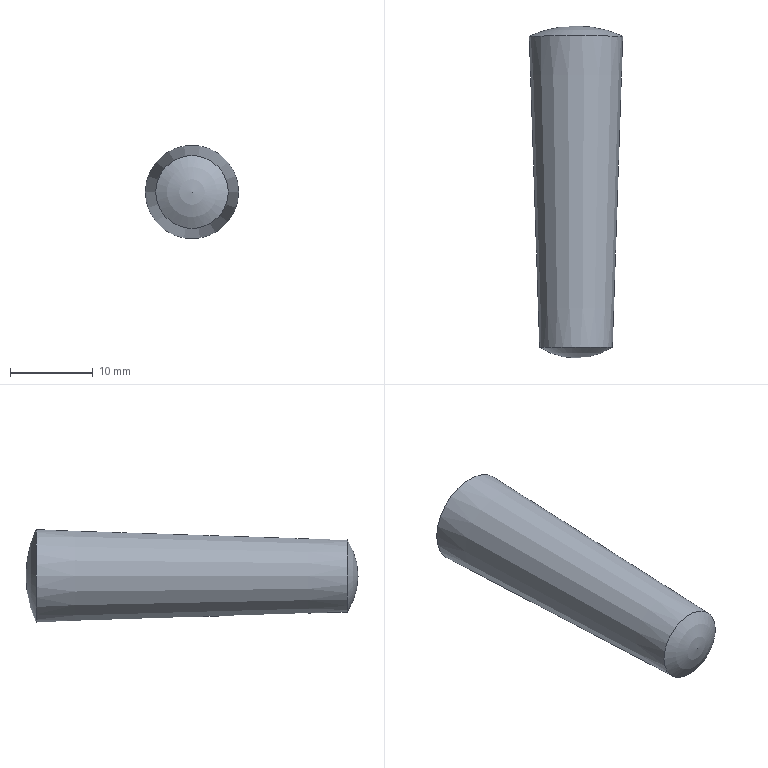Part | NX | 1 solid | 3 faces | box 11.253 x 40.001 x 11.253 mm | volume 3063 mm3 | sphere 2 | cone 1
STEP:
#1=CARTESIAN_POINT('',(-4.377,0.3088,0.));
#2=VERTEX_POINT('',#1);
#3=CARTESIAN_POINT('',(0.,0.3088,0.));
#4=DIRECTION('',(0.,1.,0.));
#5=DIRECTION('',(-1.,0.,0.));
#6=AXIS2_PLACEMENT_3D('',#3,#4,#5);
#7=CIRCLE('',#6,4.377);
#8=EDGE_CURVE('',#2,#2,#7,.T.);
#9=ORIENTED_EDGE('',*,*,#8,.F.);
#10=EDGE_LOOP('',(#9));
#11=FACE_OUTER_BOUND('',#10,.T.);
#12=CARTESIAN_POINT('',(0.,6.969,0.));
#13=DIRECTION('',(0.,1.,0.));
#14=DIRECTION('',(-1.,0.,0.));
#15=AXIS2_PLACEMENT_3D('',#12,#13,#14);
#16=SPHERICAL_SURFACE('',#15,7.97);
#17=ADVANCED_FACE('',(#11),#16,.T.);
#18=ORIENTED_EDGE('',*,*,#8,.T.);
#19=EDGE_LOOP('',(#18));
#20=FACE_BOUND('',#19,.T.);
#21=CARTESIAN_POINT('',(5.627,37.789,0.));
#22=VERTEX_POINT('',#21);
#23=CARTESIAN_POINT('',(0.,37.789,0.));
#24=DIRECTION('',(0.,1.,0.));
#25=DIRECTION('',(1.,0.,0.));
#26=AXIS2_PLACEMENT_3D('',#23,#24,#25);
#27=CIRCLE('',#26,5.627);
#28=EDGE_CURVE('',#22,#22,#27,.T.);
#29=ORIENTED_EDGE('',*,*,#28,.F.);
#30=EDGE_LOOP('',(#29));
#31=FACE_BOUND('',#30,.T.);
#32=CARTESIAN_POINT('',(0.,37.983,0.));
#33=DIRECTION('',(0.,1.,0.));
#34=DIRECTION('',(1.,0.,0.));
#35=AXIS2_PLACEMENT_3D('',#32,#33,#34);
#36=CONICAL_SURFACE('',#35,5.633,1.909);
#37=ADVANCED_FACE('',(#20,#31),#36,.T.);
#38=ORIENTED_EDGE('',*,*,#28,.T.);
#39=EDGE_LOOP('',(#38));
#40=FACE_OUTER_BOUND('',#39,.T.);
#41=CARTESIAN_POINT('',(0.,25.331,0.));
#42=DIRECTION('',(0.,1.,0.));
#43=DIRECTION('',(1.,0.,0.));
#44=AXIS2_PLACEMENT_3D('',#41,#42,#43);
#45=SPHERICAL_SURFACE('',#44,13.669);
#46=ADVANCED_FACE('',(#40),#45,.T.);
#47=CLOSED_SHELL('',(#17,#37,#46));
#48=MANIFOLD_SOLID_BREP('',#47);
#49=(LENGTH_UNIT()NAMED_UNIT(*)SI_UNIT(.MILLI.,.METRE.));
#50=UNCERTAINTY_MEASURE_WITH_UNIT(LENGTH_MEASURE(0.00002),#49,'','');
#51=(NAMED_UNIT(*)PLANE_ANGLE_UNIT()SI_UNIT($,.RADIAN.));
#52=PLANE_ANGLE_MEASURE_WITH_UNIT(PLANE_ANGLE_MEASURE(0.01745),#51);
#53=DIMENSIONAL_EXPONENTS(0.,0.,0.,0.,0.,0.,0.);
#54=(CONVERSION_BASED_UNIT('DEGREE',#52)NAMED_UNIT(#53)PLANE_ANGLE_UNIT());
#55=(NAMED_UNIT(*)SI_UNIT($,.STERADIAN.)SOLID_ANGLE_UNIT());
#56=(GEOMETRIC_REPRESENTATION_CONTEXT(3)GLOBAL_UNCERTAINTY_ASSIGNED_CONTEXT((#50))GLOBAL_UNIT_ASSIGNED_CONTEXT((#49,#54,#55))REPRESENTATION_CONTEXT('',''));
#57=ADVANCED_BREP_SHAPE_REPRESENTATION('',(#48),#56);